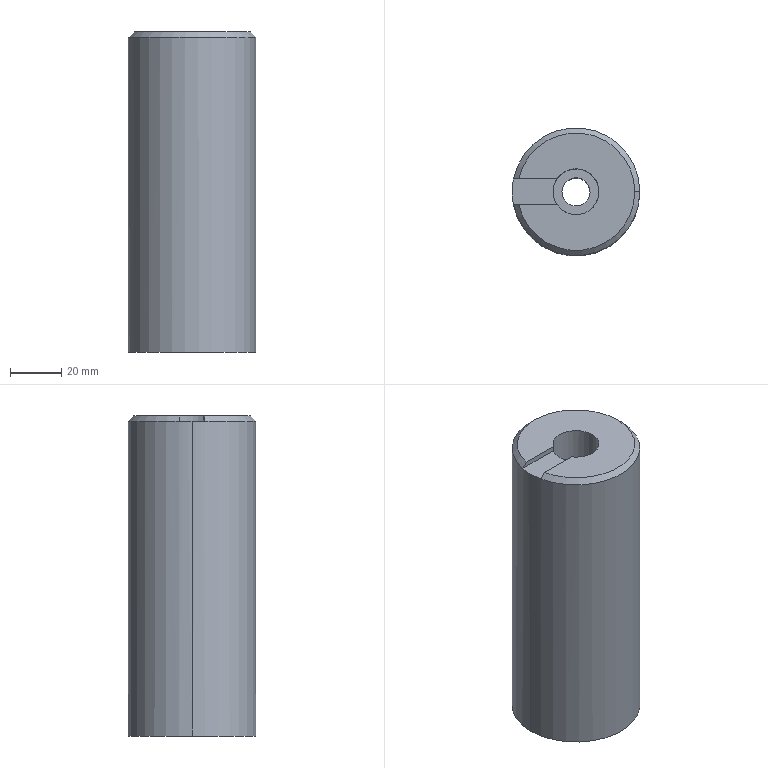Part | CATIA | 1 solid | 14 faces | box 50 x 50 x 125.3 mm | volume 227926 mm3 | plane 6 | cylinder 6 | cone 2 | commonest cylinder face diameters 11 x2 18 x2 50 x2
STEP:
#1=CARTESIAN_POINT('',(7.898,-4.315,72.3));
#2=VERTEX_POINT('',#1);
#3=CARTESIAN_POINT('',(-7.898,4.315,72.3));
#4=VERTEX_POINT('',#3);
#5=CARTESIAN_POINT('',(0.,0.,72.3));
#6=DIRECTION('',(0.,0.,-1.));
#7=AXIS2_PLACEMENT_3D('',#5,#6,$);
#8=CIRCLE('',#7,9.);
#9=EDGE_CURVE('',#2,#4,#8,.T.);
#10=ORIENTED_EDGE('',*,*,#9,.F.);
#11=CARTESIAN_POINT('',(0.,0.,72.3));
#12=DIRECTION('',(0.,0.,-1.));
#13=AXIS2_PLACEMENT_3D('',#11,#12,$);
#14=CIRCLE('',#13,9.);
#15=EDGE_CURVE('',#4,#2,#14,.T.);
#16=ORIENTED_EDGE('',*,*,#15,.F.);
#17=EDGE_LOOP('',(#10,#16));
#18=FACE_OUTER_BOUND('',#17,.T.);
#19=CARTESIAN_POINT('',(-4.827,2.637,72.3));
#20=VERTEX_POINT('',#19);
#21=CARTESIAN_POINT('',(4.827,-2.637,72.3));
#22=VERTEX_POINT('',#21);
#23=CARTESIAN_POINT('',(0.,0.,72.3));
#24=DIRECTION('',(0.,0.,-1.));
#25=AXIS2_PLACEMENT_3D('',#23,#24,$);
#26=CIRCLE('',#25,5.5);
#27=EDGE_CURVE('',#20,#22,#26,.T.);
#28=ORIENTED_EDGE('',*,*,#27,.T.);
#29=CARTESIAN_POINT('',(0.,0.,72.3));
#30=DIRECTION('',(0.,0.,-1.));
#31=AXIS2_PLACEMENT_3D('',#29,#30,$);
#32=CIRCLE('',#31,5.5);
#33=EDGE_CURVE('',#22,#20,#32,.T.);
#34=ORIENTED_EDGE('',*,*,#33,.T.);
#35=EDGE_LOOP('',(#28,#34));
#36=FACE_BOUND('',#35,.T.);
#37=CARTESIAN_POINT('',(5.5,0.,72.3));
#38=DIRECTION('',(0.,0.,-1.));
#39=DIRECTION('',(1.,0.,0.));
#40=AXIS2_PLACEMENT_3D('',#37,#38,#39);
#41=PLANE('',#40);
#42=ADVANCED_FACE('',(#18,#36),#41,.F.);
#43=CARTESIAN_POINT('',(-4.827,2.637,-18.));
#44=VERTEX_POINT('',#43);
#45=CARTESIAN_POINT('',(4.827,-2.637,-18.));
#46=VERTEX_POINT('',#45);
#47=CARTESIAN_POINT('',(0.,0.,-18.));
#48=DIRECTION('',(0.,0.,-1.));
#49=AXIS2_PLACEMENT_3D('',#47,#48,$);
#50=CIRCLE('',#49,5.5);
#51=EDGE_CURVE('',#44,#46,#50,.F.);
#52=ORIENTED_EDGE('',*,*,#51,.F.);
#53=CARTESIAN_POINT('',(-4.827,2.637,26.995));
#54=DIRECTION('',(0.,0.,-1.));
#55=VECTOR('',#54,1.);
#56=LINE('',#53,#55);
#57=EDGE_CURVE('',#44,#20,#56,.F.);
#58=ORIENTED_EDGE('',*,*,#57,.T.);
#59=ORIENTED_EDGE('',*,*,#33,.F.);
#60=CARTESIAN_POINT('',(4.827,-2.637,26.995));
#61=DIRECTION('',(0.,0.,-1.));
#62=VECTOR('',#61,1.);
#63=LINE('',#60,#62);
#64=EDGE_CURVE('',#46,#22,#63,.F.);
#65=ORIENTED_EDGE('',*,*,#64,.F.);
#66=EDGE_LOOP('',(#52,#58,#59,#65));
#67=FACE_OUTER_BOUND('',#66,.T.);
#68=CARTESIAN_POINT('',(0.,0.,107.2));
#69=DIRECTION('',(0.,0.,-1.));
#70=DIRECTION('',(0.8776,-0.4794,0.));
#71=AXIS2_PLACEMENT_3D('',#68,#69,#70);
#72=CYLINDRICAL_SURFACE('',#71,5.5);
#73=ADVANCED_FACE('',(#67),#72,.F.);
#74=CARTESIAN_POINT('',(0.,0.,-18.));
#75=DIRECTION('',(0.,0.,-1.));
#76=AXIS2_PLACEMENT_3D('',#74,#75,$);
#77=CIRCLE('',#76,5.5);
#78=EDGE_CURVE('',#46,#44,#77,.F.);
#79=ORIENTED_EDGE('',*,*,#78,.F.);
#80=ORIENTED_EDGE('',*,*,#64,.T.);
#81=ORIENTED_EDGE('',*,*,#27,.F.);
#82=ORIENTED_EDGE('',*,*,#57,.F.);
#83=EDGE_LOOP('',(#79,#80,#81,#82));
#84=FACE_OUTER_BOUND('',#83,.T.);
#85=ADVANCED_FACE('',(#84),#72,.F.);
#86=CARTESIAN_POINT('',(-7.483,5.,105.3));
#87=VERTEX_POINT('',#86);
#88=CARTESIAN_POINT('',(-24.495,5.,105.3));
#89=VERTEX_POINT('',#88);
#90=CARTESIAN_POINT('',(-15.989,5.,105.3));
#91=DIRECTION('',(1.,0.,0.));
#92=VECTOR('',#91,1.);
#93=LINE('',#90,#92);
#94=EDGE_CURVE('',#87,#89,#93,.F.);
#95=ORIENTED_EDGE('',*,*,#94,.T.);
#96=CARTESIAN_POINT('',(-25.,0.,105.3));
#97=VERTEX_POINT('',#96);
#98=CARTESIAN_POINT('',(0.,0.,105.3));
#99=DIRECTION('',(0.,0.,1.));
#100=AXIS2_PLACEMENT_3D('',#98,#99,$);
#101=CIRCLE('',#100,25.);
#102=EDGE_CURVE('',#89,#97,#101,.T.);
#103=ORIENTED_EDGE('',*,*,#102,.T.);
#104=CARTESIAN_POINT('',(-24.495,-5.,105.3));
#105=VERTEX_POINT('',#104);
#106=CARTESIAN_POINT('',(0.,0.,105.3));
#107=DIRECTION('',(0.,0.,1.));
#108=AXIS2_PLACEMENT_3D('',#106,#107,$);
#109=CIRCLE('',#108,25.);
#110=EDGE_CURVE('',#97,#105,#109,.T.);
#111=ORIENTED_EDGE('',*,*,#110,.T.);
#112=CARTESIAN_POINT('',(-7.483,-5.,105.3));
#113=VERTEX_POINT('',#112);
#114=CARTESIAN_POINT('',(-15.989,-5.,105.3));
#115=DIRECTION('',(-1.,0.,0.));
#116=VECTOR('',#115,1.);
#117=LINE('',#114,#116);
#118=EDGE_CURVE('',#105,#113,#117,.F.);
#119=ORIENTED_EDGE('',*,*,#118,.T.);
#120=CARTESIAN_POINT('',(-7.898,4.315,105.3));
#121=VERTEX_POINT('',#120);
#122=CARTESIAN_POINT('',(0.,0.,105.3));
#123=DIRECTION('',(0.,0.,1.));
#124=AXIS2_PLACEMENT_3D('',#122,#123,$);
#125=CIRCLE('',#124,9.);
#126=EDGE_CURVE('',#121,#113,#125,.T.);
#127=ORIENTED_EDGE('',*,*,#126,.F.);
#128=CARTESIAN_POINT('',(0.,0.,105.3));
#129=DIRECTION('',(0.,0.,1.));
#130=AXIS2_PLACEMENT_3D('',#128,#129,$);
#131=CIRCLE('',#130,9.);
#132=EDGE_CURVE('',#87,#121,#131,.T.);
#133=ORIENTED_EDGE('',*,*,#132,.F.);
#134=EDGE_LOOP('',(#95,#103,#111,#119,#127,#133));
#135=FACE_OUTER_BOUND('',#134,.T.);
#136=CARTESIAN_POINT('',(0.,0.,105.3));
#137=DIRECTION('',(0.,0.,1.));
#138=DIRECTION('',(1.,0.,0.));
#139=AXIS2_PLACEMENT_3D('',#136,#137,#138);
#140=PLANE('',#139);
#141=ADVANCED_FACE('',(#135),#140,.T.);
#142=CARTESIAN_POINT('',(-22.45,-5.,107.3));
#143=VERTEX_POINT('',#142);
#144=CARTESIAN_POINT('',(-7.483,-5.,107.3));
#145=VERTEX_POINT('',#144);
#146=CARTESIAN_POINT('',(-14.967,-5.,107.3));
#147=DIRECTION('',(1.,0.,0.));
#148=VECTOR('',#147,1.);
#149=LINE('',#146,#148);
#150=EDGE_CURVE('',#143,#145,#149,.T.);
#151=ORIENTED_EDGE('',*,*,#150,.F.);
#152=CARTESIAN_POINT('',(23.,0.,107.3));
#153=VERTEX_POINT('',#152);
#154=CARTESIAN_POINT('',(0.,0.,107.3));
#155=DIRECTION('',(0.,0.,1.));
#156=AXIS2_PLACEMENT_3D('',#154,#155,$);
#157=CIRCLE('',#156,23.);
#158=EDGE_CURVE('',#143,#153,#157,.T.);
#159=ORIENTED_EDGE('',*,*,#158,.T.);
#160=CARTESIAN_POINT('',(-22.45,5.,107.3));
#161=VERTEX_POINT('',#160);
#162=CARTESIAN_POINT('',(0.,0.,107.3));
#163=DIRECTION('',(0.,0.,1.));
#164=AXIS2_PLACEMENT_3D('',#162,#163,$);
#165=CIRCLE('',#164,23.);
#166=EDGE_CURVE('',#153,#161,#165,.T.);
#167=ORIENTED_EDGE('',*,*,#166,.T.);
#168=CARTESIAN_POINT('',(-7.483,5.,107.3));
#169=VERTEX_POINT('',#168);
#170=CARTESIAN_POINT('',(-14.967,5.,107.3));
#171=DIRECTION('',(1.,0.,0.));
#172=VECTOR('',#171,1.);
#173=LINE('',#170,#172);
#174=EDGE_CURVE('',#161,#169,#173,.T.);
#175=ORIENTED_EDGE('',*,*,#174,.T.);
#176=CARTESIAN_POINT('',(7.898,-4.315,107.3));
#177=VERTEX_POINT('',#176);
#178=CARTESIAN_POINT('',(0.,0.,107.3));
#179=DIRECTION('',(0.,0.,1.));
#180=AXIS2_PLACEMENT_3D('',#178,#179,$);
#181=CIRCLE('',#180,9.);
#182=EDGE_CURVE('',#177,#169,#181,.T.);
#183=ORIENTED_EDGE('',*,*,#182,.F.);
#184=CARTESIAN_POINT('',(0.,0.,107.3));
#185=DIRECTION('',(0.,0.,1.));
#186=AXIS2_PLACEMENT_3D('',#184,#185,$);
#187=CIRCLE('',#186,9.);
#188=EDGE_CURVE('',#145,#177,#187,.T.);
#189=ORIENTED_EDGE('',*,*,#188,.F.);
#190=EDGE_LOOP('',(#151,#159,#167,#175,#183,#189));
#191=FACE_OUTER_BOUND('',#190,.T.);
#192=CARTESIAN_POINT('',(0.,0.,107.3));
#193=DIRECTION('',(0.,0.,1.));
#194=DIRECTION('',(1.,0.,0.));
#195=AXIS2_PLACEMENT_3D('',#192,#193,#194);
#196=PLANE('',#195);
#197=ADVANCED_FACE('',(#191),#196,.T.);
#198=CARTESIAN_POINT('',(25.,0.,-18.));
#199=VERTEX_POINT('',#198);
#200=CARTESIAN_POINT('',(25.,0.,105.3));
#201=VERTEX_POINT('',#200);
#202=CARTESIAN_POINT('',(25.,0.,44.65));
#203=DIRECTION('',(0.,0.,1.));
#204=VECTOR('',#203,1.);
#205=LINE('',#202,#204);
#206=EDGE_CURVE('',#199,#201,#205,.T.);
#207=ORIENTED_EDGE('',*,*,#206,.F.);
#208=CARTESIAN_POINT('',(-25.,0.,-18.));
#209=VERTEX_POINT('',#208);
#210=CARTESIAN_POINT('',(0.,0.,-18.));
#211=DIRECTION('',(0.,0.,1.));
#212=AXIS2_PLACEMENT_3D('',#210,#211,$);
#213=CIRCLE('',#212,25.);
#214=EDGE_CURVE('',#199,#209,#213,.T.);
#215=ORIENTED_EDGE('',*,*,#214,.T.);
#216=CARTESIAN_POINT('',(-25.,0.,44.65));
#217=DIRECTION('',(0.,0.,1.));
#218=VECTOR('',#217,1.);
#219=LINE('',#216,#218);
#220=EDGE_CURVE('',#209,#97,#219,.T.);
#221=ORIENTED_EDGE('',*,*,#220,.T.);
#222=ORIENTED_EDGE('',*,*,#102,.F.);
#223=CARTESIAN_POINT('',(0.,0.,105.3));
#224=DIRECTION('',(0.,0.,1.));
#225=AXIS2_PLACEMENT_3D('',#223,#224,$);
#226=CIRCLE('',#225,25.);
#227=EDGE_CURVE('',#201,#89,#226,.T.);
#228=ORIENTED_EDGE('',*,*,#227,.F.);
#229=EDGE_LOOP('',(#207,#215,#221,#222,#228));
#230=FACE_OUTER_BOUND('',#229,.T.);
#231=CARTESIAN_POINT('',(0.,0.,44.65));
#232=DIRECTION('',(0.,0.,1.));
#233=DIRECTION('',(1.,0.,0.));
#234=AXIS2_PLACEMENT_3D('',#231,#232,#233);
#235=CYLINDRICAL_SURFACE('',#234,25.);
#236=ADVANCED_FACE('',(#230),#235,.T.);
#237=ORIENTED_EDGE('',*,*,#110,.F.);
#238=ORIENTED_EDGE('',*,*,#220,.F.);
#239=CARTESIAN_POINT('',(0.,0.,-18.));
#240=DIRECTION('',(0.,0.,1.));
#241=AXIS2_PLACEMENT_3D('',#239,#240,$);
#242=CIRCLE('',#241,25.);
#243=EDGE_CURVE('',#209,#199,#242,.T.);
#244=ORIENTED_EDGE('',*,*,#243,.T.);
#245=ORIENTED_EDGE('',*,*,#206,.T.);
#246=CARTESIAN_POINT('',(0.,0.,105.3));
#247=DIRECTION('',(0.,0.,1.));
#248=AXIS2_PLACEMENT_3D('',#246,#247,$);
#249=CIRCLE('',#248,25.);
#250=EDGE_CURVE('',#105,#201,#249,.T.);
#251=ORIENTED_EDGE('',*,*,#250,.F.);
#252=EDGE_LOOP('',(#237,#238,#244,#245,#251));
#253=FACE_OUTER_BOUND('',#252,.T.);
#254=ADVANCED_FACE('',(#253),#235,.T.);
#255=ORIENTED_EDGE('',*,*,#118,.F.);
#256=CARTESIAN_POINT('',(-22.45,-5.,107.3));
#257=CARTESIAN_POINT('',(-22.853,-5.,106.906));
#258=CARTESIAN_POINT('',(-23.26,-5.,106.509));
#259=CARTESIAN_POINT('',(-23.67,-5.,106.108));
#260=CARTESIAN_POINT('',(-24.081,-5.,105.705));
#261=CARTESIAN_POINT('',(-24.495,-5.,105.3));
#262=B_SPLINE_CURVE_WITH_KNOTS('',5,(#256,#257,#258,#259,#260,#261),.UNSPECIFIED.,.F.,.U.,(6,6),(0.,4.398),.UNSPECIFIED.);
#263=EDGE_CURVE('',#143,#105,#262,.T.);
#264=ORIENTED_EDGE('',*,*,#263,.F.);
#265=ORIENTED_EDGE('',*,*,#150,.T.);
#266=CARTESIAN_POINT('',(-7.483,-5.,106.3));
#267=DIRECTION('',(0.,0.,1.));
#268=VECTOR('',#267,1.);
#269=LINE('',#266,#268);
#270=EDGE_CURVE('',#113,#145,#269,.T.);
#271=ORIENTED_EDGE('',*,*,#270,.F.);
#272=EDGE_LOOP('',(#255,#264,#265,#271));
#273=FACE_OUTER_BOUND('',#272,.T.);
#274=CARTESIAN_POINT('',(0.,-5.,60.));
#275=DIRECTION('',(0.,1.,0.));
#276=DIRECTION('',(-1.,0.,0.));
#277=AXIS2_PLACEMENT_3D('',#274,#275,#276);
#278=PLANE('',#277);
#279=ADVANCED_FACE('',(#273),#278,.T.);
#280=ORIENTED_EDGE('',*,*,#263,.T.);
#281=ORIENTED_EDGE('',*,*,#250,.T.);
#282=CARTESIAN_POINT('',(24.,0.,106.3));
#283=DIRECTION('',(0.7071,0.,-0.7071));
#284=VECTOR('',#283,1.);
#285=LINE('',#282,#284);
#286=EDGE_CURVE('',#153,#201,#285,.T.);
#287=ORIENTED_EDGE('',*,*,#286,.F.);
#288=ORIENTED_EDGE('',*,*,#158,.F.);
#289=EDGE_LOOP('',(#280,#281,#287,#288));
#290=FACE_OUTER_BOUND('',#289,.T.);
#291=CARTESIAN_POINT('',(0.,0.,130.3));
#292=DIRECTION('',(0.,0.,-1.));
#293=DIRECTION('',(-0.9376,0.3478,0.));
#294=AXIS2_PLACEMENT_3D('',#291,#292,#293);
#295=CONICAL_SURFACE('',#294,0.,0.7854);
#296=ADVANCED_FACE('',(#290),#295,.T.);
#297=CARTESIAN_POINT('',(-22.45,5.,107.3));
#298=CARTESIAN_POINT('',(-23.123,5.,106.644));
#299=CARTESIAN_POINT('',(-23.805,5.,105.976));
#300=CARTESIAN_POINT('',(-24.495,5.,105.3));
#301=B_SPLINE_CURVE_WITH_KNOTS('',3,(#297,#298,#299,#300),.UNSPECIFIED.,.F.,.U.,(4,4),(0.,4.398),.UNSPECIFIED.);
#302=EDGE_CURVE('',#89,#161,#301,.F.);
#303=ORIENTED_EDGE('',*,*,#302,.T.);
#304=ORIENTED_EDGE('',*,*,#166,.F.);
#305=ORIENTED_EDGE('',*,*,#286,.T.);
#306=ORIENTED_EDGE('',*,*,#227,.T.);
#307=EDGE_LOOP('',(#303,#304,#305,#306));
#308=FACE_OUTER_BOUND('',#307,.T.);
#309=CARTESIAN_POINT('',(0.,0.,130.3));
#310=DIRECTION('',(0.,0.,-1.));
#311=DIRECTION('',(1.,0.,0.));
#312=AXIS2_PLACEMENT_3D('',#309,#310,#311);
#313=CONICAL_SURFACE('',#312,0.,0.7854);
#314=ADVANCED_FACE('',(#308),#313,.T.);
#315=ORIENTED_EDGE('',*,*,#174,.F.);
#316=ORIENTED_EDGE('',*,*,#302,.F.);
#317=ORIENTED_EDGE('',*,*,#94,.F.);
#318=CARTESIAN_POINT('',(-7.483,5.,106.3));
#319=DIRECTION('',(0.,0.,1.));
#320=VECTOR('',#319,1.);
#321=LINE('',#318,#320);
#322=EDGE_CURVE('',#87,#169,#321,.T.);
#323=ORIENTED_EDGE('',*,*,#322,.T.);
#324=EDGE_LOOP('',(#315,#316,#317,#323));
#325=FACE_OUTER_BOUND('',#324,.T.);
#326=CARTESIAN_POINT('',(-55.,5.,60.));
#327=DIRECTION('',(0.,-1.,0.));
#328=DIRECTION('',(1.,0.,0.));
#329=AXIS2_PLACEMENT_3D('',#326,#327,#328);
#330=PLANE('',#329);
#331=ADVANCED_FACE('',(#325),#330,.T.);
#332=ORIENTED_EDGE('',*,*,#243,.F.);
#333=ORIENTED_EDGE('',*,*,#214,.F.);
#334=EDGE_LOOP('',(#332,#333));
#335=FACE_OUTER_BOUND('',#334,.T.);
#336=ORIENTED_EDGE('',*,*,#78,.T.);
#337=ORIENTED_EDGE('',*,*,#51,.T.);
#338=EDGE_LOOP('',(#336,#337));
#339=FACE_BOUND('',#338,.T.);
#340=CARTESIAN_POINT('',(0.,0.,-18.));
#341=DIRECTION('',(0.,0.,1.));
#342=DIRECTION('',(1.,0.,0.));
#343=AXIS2_PLACEMENT_3D('',#340,#341,#342);
#344=PLANE('',#343);
#345=ADVANCED_FACE('',(#335,#339),#344,.F.);
#346=ORIENTED_EDGE('',*,*,#126,.T.);
#347=ORIENTED_EDGE('',*,*,#270,.T.);
#348=ORIENTED_EDGE('',*,*,#188,.T.);
#349=CARTESIAN_POINT('',(7.898,-4.315,89.955));
#350=DIRECTION('',(0.,0.,-1.));
#351=VECTOR('',#350,1.);
#352=LINE('',#349,#351);
#353=EDGE_CURVE('',#2,#177,#352,.F.);
#354=ORIENTED_EDGE('',*,*,#353,.F.);
#355=ORIENTED_EDGE('',*,*,#9,.T.);
#356=CARTESIAN_POINT('',(-7.898,4.315,89.955));
#357=DIRECTION('',(0.,0.,-1.));
#358=VECTOR('',#357,1.);
#359=LINE('',#356,#358);
#360=EDGE_CURVE('',#4,#121,#359,.F.);
#361=ORIENTED_EDGE('',*,*,#360,.T.);
#362=EDGE_LOOP('',(#346,#347,#348,#354,#355,#361));
#363=FACE_OUTER_BOUND('',#362,.T.);
#364=CARTESIAN_POINT('',(0.,0.,107.2));
#365=DIRECTION('',(0.,0.,-1.));
#366=DIRECTION('',(0.8776,-0.4794,0.));
#367=AXIS2_PLACEMENT_3D('',#364,#365,#366);
#368=CYLINDRICAL_SURFACE('',#367,9.);
#369=ADVANCED_FACE('',(#363),#368,.F.);
#370=ORIENTED_EDGE('',*,*,#182,.T.);
#371=ORIENTED_EDGE('',*,*,#322,.F.);
#372=ORIENTED_EDGE('',*,*,#132,.T.);
#373=ORIENTED_EDGE('',*,*,#360,.F.);
#374=ORIENTED_EDGE('',*,*,#15,.T.);
#375=ORIENTED_EDGE('',*,*,#353,.T.);
#376=EDGE_LOOP('',(#370,#371,#372,#373,#374,#375));
#377=FACE_OUTER_BOUND('',#376,.T.);
#378=ADVANCED_FACE('',(#377),#368,.F.);
#379=CLOSED_SHELL('',(#42,#73,#85,#141,#197,#236,#254,#279,#296,#314,#331,#345,#369,#378));
#380=MANIFOLD_SOLID_BREP('',#379);
#381=(LENGTH_UNIT()NAMED_UNIT(*)SI_UNIT(.MILLI.,.METRE.));
#382=UNCERTAINTY_MEASURE_WITH_UNIT(LENGTH_MEASURE(0.005),#381,'','');
#383=(NAMED_UNIT(*)PLANE_ANGLE_UNIT()SI_UNIT($,.RADIAN.));
#384=(NAMED_UNIT(*)SI_UNIT($,.STERADIAN.)SOLID_ANGLE_UNIT());
#385=(GEOMETRIC_REPRESENTATION_CONTEXT(3)GLOBAL_UNCERTAINTY_ASSIGNED_CONTEXT((#382))GLOBAL_UNIT_ASSIGNED_CONTEXT((#381,#383,#384))REPRESENTATION_CONTEXT('',''));
#386=ADVANCED_BREP_SHAPE_REPRESENTATION('',(#380),#385);